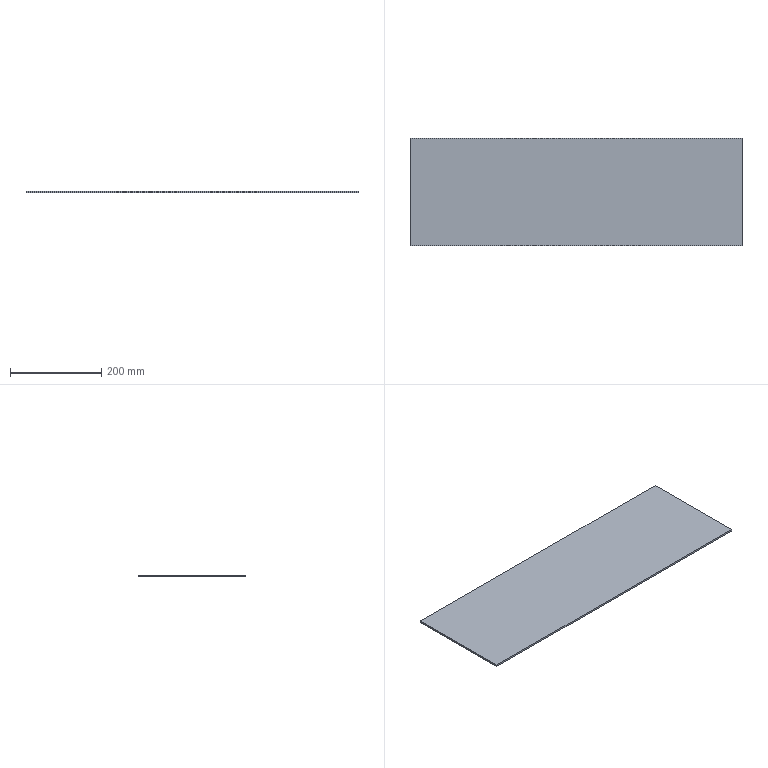Part | SolidWorks | features Extrusion 1 | 1 solid | 6 faces | box 726 x 236 x 4 mm | volume 685344 mm3 | plane 6
STEP:
#1=CARTESIAN_POINT('',(363.,-118.,0.));
#2=VERTEX_POINT('',#1);
#3=CARTESIAN_POINT('',(363.,118.,0.));
#4=VERTEX_POINT('',#3);
#5=CARTESIAN_POINT('',(363.,118.,0.));
#6=DIRECTION('',(0.,1.,0.));
#7=VECTOR('',#6,1000.);
#8=LINE('',#5,#7);
#9=EDGE_CURVE('',#2,#4,#8,.T.);
#10=ORIENTED_EDGE('',*,*,#9,.T.);
#11=CARTESIAN_POINT('',(363.,118.,4.));
#12=VERTEX_POINT('',#11);
#13=CARTESIAN_POINT('',(363.,118.,4.));
#14=DIRECTION('',(0.,0.,-1.));
#15=VECTOR('',#14,1000.);
#16=LINE('',#13,#15);
#17=EDGE_CURVE('',#12,#4,#16,.T.);
#18=ORIENTED_EDGE('',*,*,#17,.F.);
#19=CARTESIAN_POINT('',(363.,-118.,4.));
#20=VERTEX_POINT('',#19);
#21=CARTESIAN_POINT('',(363.,118.,4.));
#22=DIRECTION('',(0.,1.,0.));
#23=VECTOR('',#22,1000.);
#24=LINE('',#21,#23);
#25=EDGE_CURVE('',#20,#12,#24,.T.);
#26=ORIENTED_EDGE('',*,*,#25,.F.);
#27=CARTESIAN_POINT('',(363.,-118.,4.));
#28=DIRECTION('',(0.,0.,-1.));
#29=VECTOR('',#28,1000.);
#30=LINE('',#27,#29);
#31=EDGE_CURVE('',#20,#2,#30,.T.);
#32=ORIENTED_EDGE('',*,*,#31,.T.);
#33=EDGE_LOOP('',(#10,#18,#26,#32));
#34=FACE_OUTER_BOUND('',#33,.T.);
#35=CARTESIAN_POINT('',(363.,118.,4.));
#36=DIRECTION('',(-1.,0.,0.));
#37=DIRECTION('',(0.,-1.,0.));
#38=AXIS2_PLACEMENT_3D('',#35,#36,#37);
#39=PLANE('',#38);
#40=ADVANCED_FACE('',(#34),#39,.F.);
#41=CARTESIAN_POINT('',(-363.,118.,0.));
#42=VERTEX_POINT('',#41);
#43=CARTESIAN_POINT('',(-363.,118.,0.));
#44=DIRECTION('',(-1.,0.,0.));
#45=VECTOR('',#44,1000.);
#46=LINE('',#43,#45);
#47=EDGE_CURVE('',#4,#42,#46,.T.);
#48=ORIENTED_EDGE('',*,*,#47,.T.);
#49=CARTESIAN_POINT('',(-363.,118.,4.));
#50=VERTEX_POINT('',#49);
#51=CARTESIAN_POINT('',(-363.,118.,4.));
#52=DIRECTION('',(0.,0.,-1.));
#53=VECTOR('',#52,1000.);
#54=LINE('',#51,#53);
#55=EDGE_CURVE('',#50,#42,#54,.T.);
#56=ORIENTED_EDGE('',*,*,#55,.F.);
#57=CARTESIAN_POINT('',(-363.,118.,4.));
#58=DIRECTION('',(-1.,0.,0.));
#59=VECTOR('',#58,1000.);
#60=LINE('',#57,#59);
#61=EDGE_CURVE('',#12,#50,#60,.T.);
#62=ORIENTED_EDGE('',*,*,#61,.F.);
#63=ORIENTED_EDGE('',*,*,#17,.T.);
#64=EDGE_LOOP('',(#48,#56,#62,#63));
#65=FACE_OUTER_BOUND('',#64,.T.);
#66=CARTESIAN_POINT('',(-363.,118.,4.));
#67=DIRECTION('',(0.,-1.,0.));
#68=DIRECTION('',(0.,0.,-1.));
#69=AXIS2_PLACEMENT_3D('',#66,#67,#68);
#70=PLANE('',#69);
#71=ADVANCED_FACE('',(#65),#70,.F.);
#72=CARTESIAN_POINT('',(-363.,-118.,0.));
#73=VERTEX_POINT('',#72);
#74=CARTESIAN_POINT('',(-363.,118.,0.));
#75=DIRECTION('',(0.,-1.,0.));
#76=VECTOR('',#75,1000.);
#77=LINE('',#74,#76);
#78=EDGE_CURVE('',#42,#73,#77,.T.);
#79=ORIENTED_EDGE('',*,*,#78,.T.);
#80=CARTESIAN_POINT('',(-363.,-118.,4.));
#81=VERTEX_POINT('',#80);
#82=CARTESIAN_POINT('',(-363.,-118.,4.));
#83=DIRECTION('',(0.,0.,-1.));
#84=VECTOR('',#83,1000.);
#85=LINE('',#82,#84);
#86=EDGE_CURVE('',#81,#73,#85,.T.);
#87=ORIENTED_EDGE('',*,*,#86,.F.);
#88=CARTESIAN_POINT('',(-363.,118.,4.));
#89=DIRECTION('',(0.,-1.,0.));
#90=VECTOR('',#89,1000.);
#91=LINE('',#88,#90);
#92=EDGE_CURVE('',#50,#81,#91,.T.);
#93=ORIENTED_EDGE('',*,*,#92,.F.);
#94=ORIENTED_EDGE('',*,*,#55,.T.);
#95=EDGE_LOOP('',(#79,#87,#93,#94));
#96=FACE_OUTER_BOUND('',#95,.T.);
#97=CARTESIAN_POINT('',(-363.,118.,4.));
#98=DIRECTION('',(1.,0.,0.));
#99=DIRECTION('',(0.,0.,-1.));
#100=AXIS2_PLACEMENT_3D('',#97,#98,#99);
#101=PLANE('',#100);
#102=ADVANCED_FACE('',(#96),#101,.F.);
#103=CARTESIAN_POINT('',(-363.,-118.,0.));
#104=DIRECTION('',(1.,0.,0.));
#105=VECTOR('',#104,1000.);
#106=LINE('',#103,#105);
#107=EDGE_CURVE('',#73,#2,#106,.T.);
#108=ORIENTED_EDGE('',*,*,#107,.T.);
#109=ORIENTED_EDGE('',*,*,#31,.F.);
#110=CARTESIAN_POINT('',(-363.,-118.,4.));
#111=DIRECTION('',(1.,0.,0.));
#112=VECTOR('',#111,1000.);
#113=LINE('',#110,#112);
#114=EDGE_CURVE('',#81,#20,#113,.T.);
#115=ORIENTED_EDGE('',*,*,#114,.F.);
#116=ORIENTED_EDGE('',*,*,#86,.T.);
#117=EDGE_LOOP('',(#108,#109,#115,#116));
#118=FACE_OUTER_BOUND('',#117,.T.);
#119=CARTESIAN_POINT('',(-363.,-118.,4.));
#120=DIRECTION('',(0.,1.,0.));
#121=DIRECTION('',(0.,0.,1.));
#122=AXIS2_PLACEMENT_3D('',#119,#120,#121);
#123=PLANE('',#122);
#124=ADVANCED_FACE('',(#118),#123,.F.);
#125=ORIENTED_EDGE('',*,*,#25,.T.);
#126=ORIENTED_EDGE('',*,*,#61,.T.);
#127=ORIENTED_EDGE('',*,*,#92,.T.);
#128=ORIENTED_EDGE('',*,*,#114,.T.);
#129=EDGE_LOOP('',(#125,#126,#127,#128));
#130=FACE_OUTER_BOUND('',#129,.T.);
#131=CARTESIAN_POINT('',(0.,0.,4.));
#132=DIRECTION('',(0.,0.,1.));
#133=DIRECTION('',(1.,0.,0.));
#134=AXIS2_PLACEMENT_3D('',#131,#132,#133);
#135=PLANE('',#134);
#136=ADVANCED_FACE('',(#130),#135,.T.);
#137=ORIENTED_EDGE('',*,*,#9,.F.);
#138=ORIENTED_EDGE('',*,*,#107,.F.);
#139=ORIENTED_EDGE('',*,*,#78,.F.);
#140=ORIENTED_EDGE('',*,*,#47,.F.);
#141=EDGE_LOOP('',(#137,#138,#139,#140));
#142=FACE_OUTER_BOUND('',#141,.T.);
#143=CARTESIAN_POINT('',(0.,0.,0.));
#144=DIRECTION('',(0.,0.,1.));
#145=DIRECTION('',(1.,0.,0.));
#146=AXIS2_PLACEMENT_3D('',#143,#144,#145);
#147=PLANE('',#146);
#148=ADVANCED_FACE('',(#142),#147,.F.);
#149=CLOSED_SHELL('',(#40,#71,#102,#124,#136,#148));
#150=MANIFOLD_SOLID_BREP('',#149);
#151=CARTESIAN_POINT('',(0.,0.,0.));
#152=DIRECTION('',(0.,0.,1.));
#153=DIRECTION('',(1.,0.,0.));
#154=AXIS2_PLACEMENT_3D('',#151,#152,#153);
#155=(LENGTH_UNIT()NAMED_UNIT(*)SI_UNIT(.MILLI.,.METRE.));
#156=UNCERTAINTY_MEASURE_WITH_UNIT(LENGTH_MEASURE(0.00001),#155,'','');
#157=(NAMED_UNIT(*)PLANE_ANGLE_UNIT()SI_UNIT($,.RADIAN.));
#158=(NAMED_UNIT(*)SI_UNIT($,.STERADIAN.)SOLID_ANGLE_UNIT());
#159=(GEOMETRIC_REPRESENTATION_CONTEXT(3)GLOBAL_UNCERTAINTY_ASSIGNED_CONTEXT((#156))GLOBAL_UNIT_ASSIGNED_CONTEXT((#155,#157,#158))REPRESENTATION_CONTEXT('',''));
#160=ADVANCED_BREP_SHAPE_REPRESENTATION('',(#150,#154),#159);